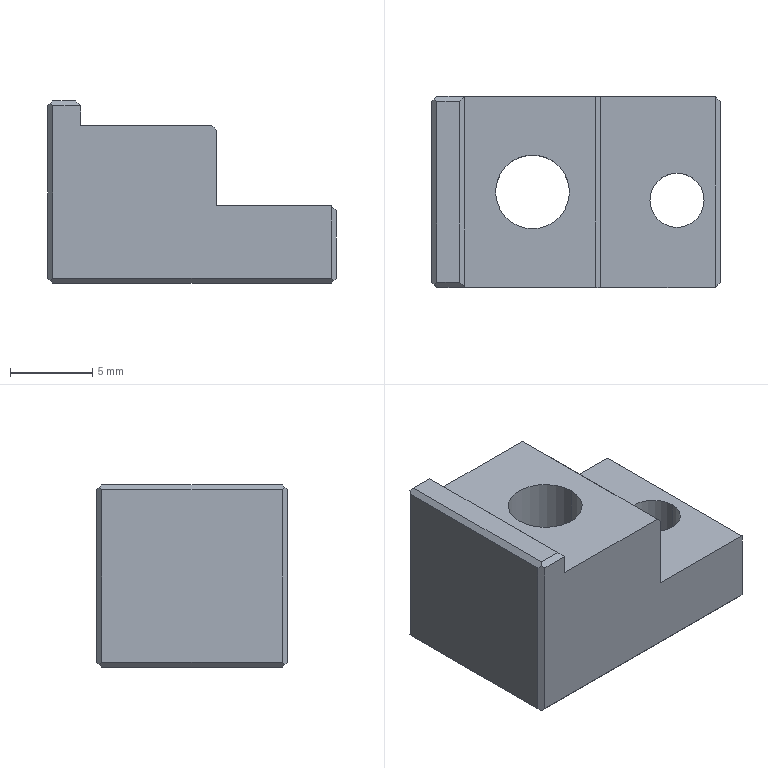Part | NX | 1 solid | 32 faces | box 17.581 x 11.62 x 11.1 mm | volume 1380 mm3 | plane 24 | cone 4 | cylinder 4 | commonest cylinder face diameters 3.3 x2 4.5 x2
STEP:
#1=CARTESIAN_POINT('',(1997.881,152.8,-124.5));
#2=VERTEX_POINT('',#1);
#3=CARTESIAN_POINT('',(1997.881,152.8,-128.6));
#4=VERTEX_POINT('',#3);
#5=CARTESIAN_POINT('',(1997.881,152.8,-126.55));
#6=DIRECTION('',(0.,0.,-1.));
#7=VECTOR('',#6,1000.);
#8=LINE('',#5,#7);
#9=EDGE_CURVE('',#2,#4,#8,.T.);
#10=ORIENTED_EDGE('',*,*,#9,.T.);
#11=CARTESIAN_POINT('',(1997.881,163.82,-128.6));
#12=VERTEX_POINT('',#11);
#13=CARTESIAN_POINT('',(1997.881,158.31,-128.6));
#14=DIRECTION('',(0.,1.,0.));
#15=VECTOR('',#14,1000.);
#16=LINE('',#13,#15);
#17=EDGE_CURVE('',#4,#12,#16,.T.);
#18=ORIENTED_EDGE('',*,*,#17,.T.);
#19=CARTESIAN_POINT('',(1997.881,163.82,-124.5));
#20=VERTEX_POINT('',#19);
#21=CARTESIAN_POINT('',(1997.881,163.82,-126.55));
#22=DIRECTION('',(0.,0.,-1.));
#23=VECTOR('',#22,1000.);
#24=LINE('',#21,#23);
#25=EDGE_CURVE('',#20,#12,#24,.T.);
#26=ORIENTED_EDGE('',*,*,#25,.F.);
#27=CARTESIAN_POINT('',(1997.881,158.31,-124.5));
#28=DIRECTION('',(0.,1.,0.));
#29=VECTOR('',#28,1000.);
#30=LINE('',#27,#29);
#31=EDGE_CURVE('',#2,#20,#30,.T.);
#32=ORIENTED_EDGE('',*,*,#31,.F.);
#33=EDGE_LOOP('',(#10,#18,#26,#32));
#34=FACE_BOUND('',#33,.T.);
#35=CARTESIAN_POINT('',(1997.881,144.5,-119.3));
#36=DIRECTION('',(1.,0.,0.));
#37=DIRECTION('',(0.,1.,0.));
#38=AXIS2_PLACEMENT_3D('',#35,#36,#37);
#39=PLANE('',#38);
#40=ADVANCED_FACE('',(#34),#39,.T.);
#41=CARTESIAN_POINT('',(1980.6,164.12,-128.6));
#42=VERTEX_POINT('',#41);
#43=CARTESIAN_POINT('',(1980.6,164.12,-118.1));
#44=VERTEX_POINT('',#43);
#45=CARTESIAN_POINT('',(1980.6,164.12,-123.35));
#46=DIRECTION('',(0.,0.,1.));
#47=VECTOR('',#46,1000.);
#48=LINE('',#45,#47);
#49=EDGE_CURVE('',#42,#44,#48,.T.);
#50=ORIENTED_EDGE('',*,*,#49,.T.);
#51=CARTESIAN_POINT('',(1982.3,164.12,-118.1));
#52=VERTEX_POINT('',#51);
#53=CARTESIAN_POINT('',(1981.3,164.12,-118.1));
#54=DIRECTION('',(-1.,0.,0.));
#55=VECTOR('',#54,1000.);
#56=LINE('',#53,#55);
#57=EDGE_CURVE('',#52,#44,#56,.T.);
#58=ORIENTED_EDGE('',*,*,#57,.F.);
#59=CARTESIAN_POINT('',(1982.3,164.12,-119.3));
#60=VERTEX_POINT('',#59);
#61=CARTESIAN_POINT('',(1982.3,164.12,-119.3));
#62=DIRECTION('',(0.,0.,1.));
#63=VECTOR('',#62,1000.);
#64=LINE('',#61,#63);
#65=EDGE_CURVE('',#60,#52,#64,.T.);
#66=ORIENTED_EDGE('',*,*,#65,.F.);
#67=CARTESIAN_POINT('',(1990.281,164.12,-119.3));
#68=VERTEX_POINT('',#67);
#69=CARTESIAN_POINT('',(1982.3,164.12,-119.3));
#70=DIRECTION('',(-1.,0.,0.));
#71=VECTOR('',#70,1000.);
#72=LINE('',#69,#71);
#73=EDGE_CURVE('',#68,#60,#72,.T.);
#74=ORIENTED_EDGE('',*,*,#73,.F.);
#75=CARTESIAN_POINT('',(1990.581,164.12,-119.6));
#76=VERTEX_POINT('',#75);
#77=CARTESIAN_POINT('',(1990.281,164.12,-119.3));
#78=DIRECTION('',(0.7071,0.,-0.7071));
#79=VECTOR('',#78,1000.);
#80=LINE('',#77,#79);
#81=EDGE_CURVE('',#68,#76,#80,.T.);
#82=ORIENTED_EDGE('',*,*,#81,.T.);
#83=CARTESIAN_POINT('',(1990.581,164.12,-124.2));
#84=VERTEX_POINT('',#83);
#85=CARTESIAN_POINT('',(1990.581,164.12,-119.3));
#86=DIRECTION('',(0.,0.,1.));
#87=VECTOR('',#86,1000.);
#88=LINE('',#85,#87);
#89=EDGE_CURVE('',#84,#76,#88,.T.);
#90=ORIENTED_EDGE('',*,*,#89,.F.);
#91=CARTESIAN_POINT('',(1997.581,164.12,-124.2));
#92=VERTEX_POINT('',#91);
#93=CARTESIAN_POINT('',(1997.8,164.12,-124.2));
#94=DIRECTION('',(-1.,0.,0.));
#95=VECTOR('',#94,1000.);
#96=LINE('',#93,#95);
#97=EDGE_CURVE('',#92,#84,#96,.T.);
#98=ORIENTED_EDGE('',*,*,#97,.F.);
#99=CARTESIAN_POINT('',(1997.581,164.12,-128.6));
#100=VERTEX_POINT('',#99);
#101=CARTESIAN_POINT('',(1997.581,164.12,-126.55));
#102=DIRECTION('',(0.,0.,-1.));
#103=VECTOR('',#102,1000.);
#104=LINE('',#101,#103);
#105=EDGE_CURVE('',#92,#100,#104,.T.);
#106=ORIENTED_EDGE('',*,*,#105,.T.);
#107=CARTESIAN_POINT('',(1989.09,164.12,-128.6));
#108=DIRECTION('',(-1.,0.,0.));
#109=VECTOR('',#108,1000.);
#110=LINE('',#107,#109);
#111=EDGE_CURVE('',#100,#42,#110,.T.);
#112=ORIENTED_EDGE('',*,*,#111,.T.);
#113=EDGE_LOOP('',(#50,#58,#66,#74,#82,#90,#98,#106,#112));
#114=FACE_BOUND('',#113,.T.);
#115=CARTESIAN_POINT('',(1980.3,164.12,-119.3));
#116=DIRECTION('',(0.,1.,0.));
#117=DIRECTION('',(1.,0.,0.));
#118=AXIS2_PLACEMENT_3D('',#115,#116,#117);
#119=PLANE('',#118);
#120=ADVANCED_FACE('',(#114),#119,.T.);
#121=CARTESIAN_POINT('',(1988.69,158.31,-128.7));
#122=VERTEX_POINT('',#121);
#123=CARTESIAN_POINT('',(1984.19,158.31,-128.7));
#124=VERTEX_POINT('',#123);
#125=CARTESIAN_POINT('',(1986.44,158.31,-128.7));
#126=DIRECTION('',(0.,0.,-1.));
#127=DIRECTION('',(-1.,0.,0.));
#128=AXIS2_PLACEMENT_3D('',#125,#126,#127);
#129=CIRCLE('',#128,2.25);
#130=EDGE_CURVE('',#122,#124,#129,.T.);
#131=ORIENTED_EDGE('',*,*,#130,.F.);
#132=CARTESIAN_POINT('',(1988.89,158.31,-128.9));
#133=VERTEX_POINT('',#132);
#134=CARTESIAN_POINT('',(1988.69,158.31,-128.7));
#135=DIRECTION('',(0.7071,0.,-0.7071));
#136=VECTOR('',#135,1000.);
#137=LINE('',#134,#136);
#138=EDGE_CURVE('',#133,#122,#137,.F.);
#139=ORIENTED_EDGE('',*,*,#138,.F.);
#140=CARTESIAN_POINT('',(1983.99,158.31,-128.9));
#141=VERTEX_POINT('',#140);
#142=CARTESIAN_POINT('',(1986.44,158.31,-128.9));
#143=DIRECTION('',(0.,0.,-1.));
#144=DIRECTION('',(-1.,0.,0.));
#145=AXIS2_PLACEMENT_3D('',#142,#143,#144);
#146=CIRCLE('',#145,2.45);
#147=EDGE_CURVE('',#133,#141,#146,.T.);
#148=ORIENTED_EDGE('',*,*,#147,.T.);
#149=CARTESIAN_POINT('',(1984.19,158.31,-128.7));
#150=DIRECTION('',(-0.7071,0.,-0.7071));
#151=VECTOR('',#150,1000.);
#152=LINE('',#149,#151);
#153=EDGE_CURVE('',#141,#124,#152,.F.);
#154=ORIENTED_EDGE('',*,*,#153,.T.);
#155=EDGE_LOOP('',(#131,#139,#148,#154));
#156=FACE_BOUND('',#155,.T.);
#157=CARTESIAN_POINT('',(1986.44,158.31,-128.7));
#158=DIRECTION('',(0.,0.,-1.));
#159=DIRECTION('',(-1.,0.,0.));
#160=AXIS2_PLACEMENT_3D('',#157,#158,#159);
#161=CONICAL_SURFACE('',#160,2.25,0.7854);
#162=ADVANCED_FACE('',(#156),#161,.F.);
#163=CARTESIAN_POINT('',(1982.3,152.5,-119.3));
#164=VERTEX_POINT('',#163);
#165=CARTESIAN_POINT('',(1982.3,152.5,-118.1));
#166=VERTEX_POINT('',#165);
#167=CARTESIAN_POINT('',(1982.3,152.5,-119.3));
#168=DIRECTION('',(0.,0.,1.));
#169=VECTOR('',#168,1000.);
#170=LINE('',#167,#169);
#171=EDGE_CURVE('',#164,#166,#170,.T.);
#172=ORIENTED_EDGE('',*,*,#171,.T.);
#173=CARTESIAN_POINT('',(1980.6,152.5,-118.1));
#174=VERTEX_POINT('',#173);
#175=CARTESIAN_POINT('',(1981.3,152.5,-118.1));
#176=DIRECTION('',(1.,0.,0.));
#177=VECTOR('',#176,1000.);
#178=LINE('',#175,#177);
#179=EDGE_CURVE('',#174,#166,#178,.T.);
#180=ORIENTED_EDGE('',*,*,#179,.F.);
#181=CARTESIAN_POINT('',(1980.6,152.5,-128.6));
#182=VERTEX_POINT('',#181);
#183=CARTESIAN_POINT('',(1980.6,152.5,-123.35));
#184=DIRECTION('',(0.,0.,1.));
#185=VECTOR('',#184,1000.);
#186=LINE('',#183,#185);
#187=EDGE_CURVE('',#182,#174,#186,.T.);
#188=ORIENTED_EDGE('',*,*,#187,.F.);
#189=CARTESIAN_POINT('',(1997.581,152.5,-128.6));
#190=VERTEX_POINT('',#189);
#191=CARTESIAN_POINT('',(1989.09,152.5,-128.6));
#192=DIRECTION('',(-1.,0.,0.));
#193=VECTOR('',#192,1000.);
#194=LINE('',#191,#193);
#195=EDGE_CURVE('',#190,#182,#194,.T.);
#196=ORIENTED_EDGE('',*,*,#195,.F.);
#197=CARTESIAN_POINT('',(1997.581,152.5,-124.2));
#198=VERTEX_POINT('',#197);
#199=CARTESIAN_POINT('',(1997.581,152.5,-126.55));
#200=DIRECTION('',(0.,0.,-1.));
#201=VECTOR('',#200,1000.);
#202=LINE('',#199,#201);
#203=EDGE_CURVE('',#198,#190,#202,.T.);
#204=ORIENTED_EDGE('',*,*,#203,.F.);
#205=CARTESIAN_POINT('',(1990.581,152.5,-124.2));
#206=VERTEX_POINT('',#205);
#207=CARTESIAN_POINT('',(1997.8,152.5,-124.2));
#208=DIRECTION('',(1.,0.,0.));
#209=VECTOR('',#208,1000.);
#210=LINE('',#207,#209);
#211=EDGE_CURVE('',#206,#198,#210,.T.);
#212=ORIENTED_EDGE('',*,*,#211,.F.);
#213=CARTESIAN_POINT('',(1990.581,152.5,-119.6));
#214=VERTEX_POINT('',#213);
#215=CARTESIAN_POINT('',(1990.581,152.5,-119.3));
#216=DIRECTION('',(0.,0.,-1.));
#217=VECTOR('',#216,1000.);
#218=LINE('',#215,#217);
#219=EDGE_CURVE('',#214,#206,#218,.T.);
#220=ORIENTED_EDGE('',*,*,#219,.F.);
#221=CARTESIAN_POINT('',(1990.281,152.5,-119.3));
#222=VERTEX_POINT('',#221);
#223=CARTESIAN_POINT('',(1990.281,152.5,-119.3));
#224=DIRECTION('',(-0.7071,0.,0.7071));
#225=VECTOR('',#224,1000.);
#226=LINE('',#223,#225);
#227=EDGE_CURVE('',#214,#222,#226,.T.);
#228=ORIENTED_EDGE('',*,*,#227,.T.);
#229=CARTESIAN_POINT('',(1988.678,152.5,-119.3));
#230=DIRECTION('',(-1.,0.,0.));
#231=VECTOR('',#230,1000.);
#232=LINE('',#229,#231);
#233=EDGE_CURVE('',#222,#164,#232,.T.);
#234=ORIENTED_EDGE('',*,*,#233,.T.);
#235=EDGE_LOOP('',(#172,#180,#188,#196,#204,#212,#220,#228,#234));
#236=FACE_BOUND('',#235,.T.);
#237=CARTESIAN_POINT('',(1982.3,152.5,-119.3));
#238=DIRECTION('',(0.,-1.,0.));
#239=DIRECTION('',(0.,0.,-1.));
#240=AXIS2_PLACEMENT_3D('',#237,#238,#239);
#241=PLANE('',#240);
#242=ADVANCED_FACE('',(#236),#241,.T.);
#243=ORIENTED_EDGE('',*,*,#130,.T.);
#244=CARTESIAN_POINT('',(1984.19,158.31,-119.3));
#245=VERTEX_POINT('',#244);
#246=CARTESIAN_POINT('',(1984.19,158.31,-128.9));
#247=DIRECTION('',(0.,0.,-1.));
#248=VECTOR('',#247,1000.);
#249=LINE('',#246,#248);
#250=EDGE_CURVE('',#124,#245,#249,.F.);
#251=ORIENTED_EDGE('',*,*,#250,.T.);
#252=CARTESIAN_POINT('',(1988.69,158.31,-119.3));
#253=VERTEX_POINT('',#252);
#254=CARTESIAN_POINT('',(1986.44,158.31,-119.3));
#255=DIRECTION('',(0.,0.,-1.));
#256=DIRECTION('',(-1.,0.,0.));
#257=AXIS2_PLACEMENT_3D('',#254,#255,#256);
#258=CIRCLE('',#257,2.25);
#259=EDGE_CURVE('',#253,#245,#258,.T.);
#260=ORIENTED_EDGE('',*,*,#259,.F.);
#261=CARTESIAN_POINT('',(1988.69,158.31,-128.9));
#262=DIRECTION('',(0.,0.,-1.));
#263=VECTOR('',#262,1000.);
#264=LINE('',#261,#263);
#265=EDGE_CURVE('',#122,#253,#264,.F.);
#266=ORIENTED_EDGE('',*,*,#265,.F.);
#267=EDGE_LOOP('',(#243,#251,#260,#266));
#268=FACE_BOUND('',#267,.T.);
#269=CARTESIAN_POINT('',(1986.44,158.31,-128.9));
#270=DIRECTION('',(0.,0.,-1.));
#271=DIRECTION('',(-1.,0.,0.));
#272=AXIS2_PLACEMENT_3D('',#269,#270,#271);
#273=CYLINDRICAL_SURFACE('',#272,2.25);
#274=ADVANCED_FACE('',(#268),#273,.F.);
#275=CARTESIAN_POINT('',(1982.,163.82,-117.8));
#276=VERTEX_POINT('',#275);
#277=CARTESIAN_POINT('',(1980.6,163.82,-117.8));
#278=VERTEX_POINT('',#277);
#279=CARTESIAN_POINT('',(1981.3,163.82,-117.8));
#280=DIRECTION('',(-1.,0.,0.));
#281=VECTOR('',#280,1000.);
#282=LINE('',#279,#281);
#283=EDGE_CURVE('',#276,#278,#282,.T.);
#284=ORIENTED_EDGE('',*,*,#283,.T.);
#285=CARTESIAN_POINT('',(1980.6,152.8,-117.8));
#286=VERTEX_POINT('',#285);
#287=CARTESIAN_POINT('',(1980.6,158.31,-117.8));
#288=DIRECTION('',(0.,-1.,0.));
#289=VECTOR('',#288,1000.);
#290=LINE('',#287,#289);
#291=EDGE_CURVE('',#278,#286,#290,.T.);
#292=ORIENTED_EDGE('',*,*,#291,.T.);
#293=CARTESIAN_POINT('',(1982.,152.8,-117.8));
#294=VERTEX_POINT('',#293);
#295=CARTESIAN_POINT('',(1981.3,152.8,-117.8));
#296=DIRECTION('',(1.,0.,0.));
#297=VECTOR('',#296,1000.);
#298=LINE('',#295,#297);
#299=EDGE_CURVE('',#286,#294,#298,.T.);
#300=ORIENTED_EDGE('',*,*,#299,.T.);
#301=CARTESIAN_POINT('',(1982.,158.31,-117.8));
#302=DIRECTION('',(0.,1.,0.));
#303=VECTOR('',#302,1000.);
#304=LINE('',#301,#303);
#305=EDGE_CURVE('',#294,#276,#304,.T.);
#306=ORIENTED_EDGE('',*,*,#305,.T.);
#307=EDGE_LOOP('',(#284,#292,#300,#306));
#308=FACE_BOUND('',#307,.T.);
#309=CARTESIAN_POINT('',(1989.636,158.31,-117.8));
#310=DIRECTION('',(0.,0.,1.));
#311=DIRECTION('',(1.,0.,0.));
#312=AXIS2_PLACEMENT_3D('',#309,#310,#311);
#313=PLANE('',#312);
#314=ADVANCED_FACE('',(#308),#313,.T.);
#315=CARTESIAN_POINT('',(1982.3,148.25,-119.3));
#316=DIRECTION('',(0.,-1.,0.));
#317=VECTOR('',#316,1000.);
#318=LINE('',#315,#317);
#319=EDGE_CURVE('',#60,#164,#318,.T.);
#320=ORIENTED_EDGE('',*,*,#319,.F.);
#321=ORIENTED_EDGE('',*,*,#65,.T.);
#322=CARTESIAN_POINT('',(1982.3,158.31,-118.1));
#323=DIRECTION('',(0.,1.,0.));
#324=VECTOR('',#323,1000.);
#325=LINE('',#322,#324);
#326=EDGE_CURVE('',#166,#52,#325,.T.);
#327=ORIENTED_EDGE('',*,*,#326,.F.);
#328=ORIENTED_EDGE('',*,*,#171,.F.);
#329=EDGE_LOOP('',(#320,#321,#327,#328));
#330=FACE_BOUND('',#329,.T.);
#331=CARTESIAN_POINT('',(1982.3,164.12,-119.3));
#332=DIRECTION('',(1.,0.,0.));
#333=DIRECTION('',(0.,1.,0.));
#334=AXIS2_PLACEMENT_3D('',#331,#332,#333);
#335=PLANE('',#334);
#336=ADVANCED_FACE('',(#330),#335,.T.);
#337=ORIENTED_EDGE('',*,*,#111,.F.);
#338=CARTESIAN_POINT('',(1997.731,163.97,-128.75));
#339=VERTEX_POINT('',#338);
#340=CARTESIAN_POINT('',(1988.281,173.42,-119.3));
#341=DIRECTION('',(-0.5774,0.5774,0.5774));
#342=VECTOR('',#341,1000.);
#343=LINE('',#340,#342);
#344=EDGE_CURVE('',#339,#100,#343,.T.);
#345=ORIENTED_EDGE('',*,*,#344,.F.);
#346=CARTESIAN_POINT('',(1997.581,163.82,-128.9));
#347=VERTEX_POINT('',#346);
#348=CARTESIAN_POINT('',(2007.181,173.42,-119.3));
#349=DIRECTION('',(0.5774,0.5774,0.5774));
#350=VECTOR('',#349,1000.);
#351=LINE('',#348,#350);
#352=EDGE_CURVE('',#347,#339,#351,.T.);
#353=ORIENTED_EDGE('',*,*,#352,.F.);
#354=CARTESIAN_POINT('',(1980.6,163.82,-128.9));
#355=VERTEX_POINT('',#354);
#356=CARTESIAN_POINT('',(1989.09,163.82,-128.9));
#357=DIRECTION('',(-1.,0.,0.));
#358=VECTOR('',#357,1000.);
#359=LINE('',#356,#358);
#360=EDGE_CURVE('',#347,#355,#359,.T.);
#361=ORIENTED_EDGE('',*,*,#360,.T.);
#362=CARTESIAN_POINT('',(1980.45,163.97,-128.75));
#363=VERTEX_POINT('',#362);
#364=CARTESIAN_POINT('',(1971.,173.42,-119.3));
#365=DIRECTION('',(-0.5774,0.5774,0.5774));
#366=VECTOR('',#365,1000.);
#367=LINE('',#364,#366);
#368=EDGE_CURVE('',#355,#363,#367,.T.);
#369=ORIENTED_EDGE('',*,*,#368,.T.);
#370=CARTESIAN_POINT('',(1989.9,173.42,-119.3));
#371=DIRECTION('',(0.5774,0.5774,0.5774));
#372=VECTOR('',#371,1000.);
#373=LINE('',#370,#372);
#374=EDGE_CURVE('',#363,#42,#373,.T.);
#375=ORIENTED_EDGE('',*,*,#374,.T.);
#376=EDGE_LOOP('',(#337,#345,#353,#361,#369,#375));
#377=FACE_BOUND('',#376,.T.);
#378=CARTESIAN_POINT('',(1989.09,163.97,-128.75));
#379=DIRECTION('',(0.,0.7071,-0.7071));
#380=DIRECTION('',(-1.,0.,0.));
#381=AXIS2_PLACEMENT_3D('',#378,#379,#380);
#382=PLANE('',#381);
#383=ADVANCED_FACE('',(#377),#382,.T.);
#384=ORIENTED_EDGE('',*,*,#25,.T.);
#385=CARTESIAN_POINT('',(2013.451,148.25,-113.03));
#386=DIRECTION('',(-0.5774,0.5774,-0.5774));
#387=VECTOR('',#386,1000.);
#388=LINE('',#385,#387);
#389=EDGE_CURVE('',#12,#339,#388,.T.);
#390=ORIENTED_EDGE('',*,*,#389,.T.);
#391=ORIENTED_EDGE('',*,*,#344,.T.);
#392=ORIENTED_EDGE('',*,*,#105,.F.);
#393=CARTESIAN_POINT('',(2013.451,148.25,-140.07));
#394=DIRECTION('',(0.5774,-0.5774,-0.5774));
#395=VECTOR('',#394,1000.);
#396=LINE('',#393,#395);
#397=EDGE_CURVE('',#92,#20,#396,.T.);
#398=ORIENTED_EDGE('',*,*,#397,.T.);
#399=EDGE_LOOP('',(#384,#390,#391,#392,#398));
#400=FACE_BOUND('',#399,.T.);
#401=CARTESIAN_POINT('',(1997.731,163.97,-126.55));
#402=DIRECTION('',(-0.7071,-0.7071,0.));
#403=DIRECTION('',(-0.7071,0.7071,0.));
#404=AXIS2_PLACEMENT_3D('',#401,#402,#403);
#405=PLANE('',#404);
#406=ADVANCED_FACE('',(#400),#405,.F.);
#407=ORIENTED_EDGE('',*,*,#9,.F.);
#408=CARTESIAN_POINT('',(1992.681,147.6,-119.3));
#409=DIRECTION('',(0.5774,0.5774,-0.5774));
#410=VECTOR('',#409,1000.);
#411=LINE('',#408,#410);
#412=EDGE_CURVE('',#198,#2,#411,.T.);
#413=ORIENTED_EDGE('',*,*,#412,.F.);
#414=ORIENTED_EDGE('',*,*,#203,.T.);
#415=CARTESIAN_POINT('',(1997.731,152.65,-128.75));
#416=VERTEX_POINT('',#415);
#417=CARTESIAN_POINT('',(1988.281,143.2,-119.3));
#418=DIRECTION('',(0.5774,0.5774,-0.5774));
#419=VECTOR('',#418,1000.);
#420=LINE('',#417,#419);
#421=EDGE_CURVE('',#190,#416,#420,.T.);
#422=ORIENTED_EDGE('',*,*,#421,.T.);
#423=CARTESIAN_POINT('',(2007.181,162.1,-119.3));
#424=DIRECTION('',(0.5774,0.5774,0.5774));
#425=VECTOR('',#424,1000.);
#426=LINE('',#423,#425);
#427=EDGE_CURVE('',#416,#4,#426,.T.);
#428=ORIENTED_EDGE('',*,*,#427,.T.);
#429=EDGE_LOOP('',(#407,#413,#414,#422,#428));
#430=FACE_BOUND('',#429,.T.);
#431=CARTESIAN_POINT('',(1997.731,152.65,-126.55));
#432=DIRECTION('',(0.7071,-0.7071,0.));
#433=DIRECTION('',(0.,0.,-1.));
#434=AXIS2_PLACEMENT_3D('',#431,#432,#433);
#435=PLANE('',#434);
#436=ADVANCED_FACE('',(#430),#435,.T.);
#437=ORIENTED_EDGE('',*,*,#49,.F.);
#438=ORIENTED_EDGE('',*,*,#374,.F.);
#439=CARTESIAN_POINT('',(1980.3,163.82,-128.6));
#440=VERTEX_POINT('',#439);
#441=CARTESIAN_POINT('',(1971.,154.52,-119.3));
#442=DIRECTION('',(0.5774,0.5774,-0.5774));
#443=VECTOR('',#442,1000.);
#444=LINE('',#441,#443);
#445=EDGE_CURVE('',#440,#363,#444,.T.);
#446=ORIENTED_EDGE('',*,*,#445,.F.);
#447=CARTESIAN_POINT('',(1980.3,163.82,-118.1));
#448=VERTEX_POINT('',#447);
#449=CARTESIAN_POINT('',(1980.3,163.82,-123.35));
#450=DIRECTION('',(0.,0.,1.));
#451=VECTOR('',#450,1000.);
#452=LINE('',#449,#451);
#453=EDGE_CURVE('',#440,#448,#452,.T.);
#454=ORIENTED_EDGE('',*,*,#453,.T.);
#455=CARTESIAN_POINT('',(1980.45,163.97,-117.95));
#456=VERTEX_POINT('',#455);
#457=CARTESIAN_POINT('',(1997.8,181.32,-100.6));
#458=DIRECTION('',(0.5774,0.5774,0.5774));
#459=VECTOR('',#458,1000.);
#460=LINE('',#457,#459);
#461=EDGE_CURVE('',#448,#456,#460,.T.);
#462=ORIENTED_EDGE('',*,*,#461,.T.);
#463=CARTESIAN_POINT('',(1964.73,148.25,-102.23));
#464=DIRECTION('',(0.5774,0.5774,-0.5774));
#465=VECTOR('',#464,1000.);
#466=LINE('',#463,#465);
#467=EDGE_CURVE('',#456,#44,#466,.T.);
#468=ORIENTED_EDGE('',*,*,#467,.T.);
#469=EDGE_LOOP('',(#437,#438,#446,#454,#462,#468));
#470=FACE_BOUND('',#469,.T.);
#471=CARTESIAN_POINT('',(1980.45,163.97,-123.35));
#472=DIRECTION('',(-0.7071,0.7071,0.));
#473=DIRECTION('',(0.,0.,1.));
#474=AXIS2_PLACEMENT_3D('',#471,#472,#473);
#475=PLANE('',#474);
#476=ADVANCED_FACE('',(#470),#475,.T.);
#477=ORIENTED_EDGE('',*,*,#291,.F.);
#478=CARTESIAN_POINT('',(1996.17,148.25,-102.23));
#479=DIRECTION('',(-0.5774,0.5774,-0.5774));
#480=VECTOR('',#479,1000.);
#481=LINE('',#478,#480);
#482=EDGE_CURVE('',#278,#456,#481,.T.);
#483=ORIENTED_EDGE('',*,*,#482,.T.);
#484=ORIENTED_EDGE('',*,*,#461,.F.);
#485=CARTESIAN_POINT('',(1980.3,152.8,-118.1));
#486=VERTEX_POINT('',#485);
#487=CARTESIAN_POINT('',(1980.3,158.31,-118.1));
#488=DIRECTION('',(0.,-1.,0.));
#489=VECTOR('',#488,1000.);
#490=LINE('',#487,#489);
#491=EDGE_CURVE('',#448,#486,#490,.T.);
#492=ORIENTED_EDGE('',*,*,#491,.T.);
#493=CARTESIAN_POINT('',(1980.45,152.65,-117.95));
#494=VERTEX_POINT('',#493);
#495=CARTESIAN_POINT('',(1997.8,135.3,-100.6));
#496=DIRECTION('',(-0.5774,0.5774,-0.5774));
#497=VECTOR('',#496,1000.);
#498=LINE('',#495,#497);
#499=EDGE_CURVE('',#494,#486,#498,.T.);
#500=ORIENTED_EDGE('',*,*,#499,.F.);
#501=CARTESIAN_POINT('',(1997.8,170.,-100.6));
#502=DIRECTION('',(0.5774,0.5774,0.5774));
#503=VECTOR('',#502,1000.);
#504=LINE('',#501,#503);
#505=EDGE_CURVE('',#494,#286,#504,.T.);
#506=ORIENTED_EDGE('',*,*,#505,.T.);
#507=EDGE_LOOP('',(#477,#483,#484,#492,#500,#506));
#508=FACE_BOUND('',#507,.T.);
#509=CARTESIAN_POINT('',(1980.45,158.31,-117.95));
#510=DIRECTION('',(-0.7071,0.,0.7071));
#511=DIRECTION('',(0.,1.,0.));
#512=AXIS2_PLACEMENT_3D('',#509,#510,#511);
#513=PLANE('',#512);
#514=ADVANCED_FACE('',(#508),#513,.T.);
#515=ORIENTED_EDGE('',*,*,#305,.F.);
#516=CARTESIAN_POINT('',(1997.8,137.,-133.6));
#517=DIRECTION('',(0.5774,-0.5774,-0.5774));
#518=VECTOR('',#517,1000.);
#519=LINE('',#516,#518);
#520=EDGE_CURVE('',#294,#166,#519,.T.);
#521=ORIENTED_EDGE('',*,*,#520,.T.);
#522=ORIENTED_EDGE('',*,*,#326,.T.);
#523=CARTESIAN_POINT('',(1966.43,148.25,-102.23));
#524=DIRECTION('',(-0.5774,-0.5774,0.5774));
#525=VECTOR('',#524,1000.);
#526=LINE('',#523,#525);
#527=EDGE_CURVE('',#52,#276,#526,.T.);
#528=ORIENTED_EDGE('',*,*,#527,.T.);
#529=EDGE_LOOP('',(#515,#521,#522,#528));
#530=FACE_BOUND('',#529,.T.);
#531=CARTESIAN_POINT('',(1982.15,158.31,-117.95));
#532=DIRECTION('',(0.7071,0.,0.7071));
#533=DIRECTION('',(0.,-1.,0.));
#534=AXIS2_PLACEMENT_3D('',#531,#532,#533);
#535=PLANE('',#534);
#536=ADVANCED_FACE('',(#530),#535,.T.);
#537=ORIENTED_EDGE('',*,*,#299,.F.);
#538=ORIENTED_EDGE('',*,*,#505,.F.);
#539=CARTESIAN_POINT('',(1981.8,151.3,-119.3));
#540=DIRECTION('',(-0.5774,0.5774,0.5774));
#541=VECTOR('',#540,1000.);
#542=LINE('',#539,#541);
#543=EDGE_CURVE('',#174,#494,#542,.T.);
#544=ORIENTED_EDGE('',*,*,#543,.F.);
#545=ORIENTED_EDGE('',*,*,#179,.T.);
#546=ORIENTED_EDGE('',*,*,#520,.F.);
#547=EDGE_LOOP('',(#537,#538,#544,#545,#546));
#548=FACE_BOUND('',#547,.T.);
#549=CARTESIAN_POINT('',(1981.3,152.65,-117.95));
#550=DIRECTION('',(0.,-0.7071,0.7071));
#551=DIRECTION('',(-1.,0.,0.));
#552=AXIS2_PLACEMENT_3D('',#549,#550,#551);
#553=PLANE('',#552);
#554=ADVANCED_FACE('',(#548),#553,.T.);
#555=ORIENTED_EDGE('',*,*,#283,.F.);
#556=ORIENTED_EDGE('',*,*,#527,.F.);
#557=ORIENTED_EDGE('',*,*,#57,.T.);
#558=ORIENTED_EDGE('',*,*,#467,.F.);
#559=ORIENTED_EDGE('',*,*,#482,.F.);
#560=EDGE_LOOP('',(#555,#556,#557,#558,#559));
#561=FACE_BOUND('',#560,.T.);
#562=CARTESIAN_POINT('',(1981.3,163.97,-117.95));
#563=DIRECTION('',(0.,0.7071,0.7071));
#564=DIRECTION('',(1.,0.,0.));
#565=AXIS2_PLACEMENT_3D('',#562,#563,#564);
#566=PLANE('',#565);
#567=ADVANCED_FACE('',(#561),#566,.T.);
#568=ORIENTED_EDGE('',*,*,#153,.F.);
#569=CARTESIAN_POINT('',(1986.44,158.31,-128.9));
#570=DIRECTION('',(0.,0.,-1.));
#571=DIRECTION('',(-1.,0.,0.));
#572=AXIS2_PLACEMENT_3D('',#569,#570,#571);
#573=CIRCLE('',#572,2.45);
#574=EDGE_CURVE('',#141,#133,#573,.T.);
#575=ORIENTED_EDGE('',*,*,#574,.T.);
#576=ORIENTED_EDGE('',*,*,#138,.T.);
#577=CARTESIAN_POINT('',(1986.44,158.31,-128.7));
#578=DIRECTION('',(0.,0.,-1.));
#579=DIRECTION('',(-1.,0.,0.));
#580=AXIS2_PLACEMENT_3D('',#577,#578,#579);
#581=CIRCLE('',#580,2.25);
#582=EDGE_CURVE('',#124,#122,#581,.T.);
#583=ORIENTED_EDGE('',*,*,#582,.F.);
#584=EDGE_LOOP('',(#568,#575,#576,#583));
#585=FACE_BOUND('',#584,.T.);
#586=CARTESIAN_POINT('',(1986.44,158.31,-128.7));
#587=DIRECTION('',(0.,0.,-1.));
#588=DIRECTION('',(-1.,0.,0.));
#589=AXIS2_PLACEMENT_3D('',#586,#587,#588);
#590=CONICAL_SURFACE('',#589,2.25,0.7854);
#591=ADVANCED_FACE('',(#585),#590,.F.);
#592=ORIENTED_EDGE('',*,*,#250,.F.);
#593=ORIENTED_EDGE('',*,*,#582,.T.);
#594=ORIENTED_EDGE('',*,*,#265,.T.);
#595=CARTESIAN_POINT('',(1986.44,158.31,-119.3));
#596=DIRECTION('',(0.,0.,-1.));
#597=DIRECTION('',(-1.,0.,0.));
#598=AXIS2_PLACEMENT_3D('',#595,#596,#597);
#599=CIRCLE('',#598,2.25);
#600=EDGE_CURVE('',#245,#253,#599,.T.);
#601=ORIENTED_EDGE('',*,*,#600,.F.);
#602=EDGE_LOOP('',(#592,#593,#594,#601));
#603=FACE_BOUND('',#602,.T.);
#604=CARTESIAN_POINT('',(1986.44,158.31,-128.9));
#605=DIRECTION('',(0.,0.,-1.));
#606=DIRECTION('',(-1.,0.,0.));
#607=AXIS2_PLACEMENT_3D('',#604,#605,#606);
#608=CYLINDRICAL_SURFACE('',#607,2.25);
#609=ADVANCED_FACE('',(#603),#608,.F.);
#610=CARTESIAN_POINT('',(1997.581,152.8,-128.9));
#611=VERTEX_POINT('',#610);
#612=CARTESIAN_POINT('',(1980.6,152.8,-128.9));
#613=VERTEX_POINT('',#612);
#614=CARTESIAN_POINT('',(1989.09,152.8,-128.9));
#615=DIRECTION('',(-1.,0.,0.));
#616=VECTOR('',#615,1000.);
#617=LINE('',#614,#616);
#618=EDGE_CURVE('',#611,#613,#617,.T.);
#619=ORIENTED_EDGE('',*,*,#618,.T.);
#620=CARTESIAN_POINT('',(1980.6,158.31,-128.9));
#621=DIRECTION('',(0.,-1.,0.));
#622=VECTOR('',#621,1000.);
#623=LINE('',#620,#622);
#624=EDGE_CURVE('',#355,#613,#623,.T.);
#625=ORIENTED_EDGE('',*,*,#624,.F.);
#626=ORIENTED_EDGE('',*,*,#360,.F.);
#627=CARTESIAN_POINT('',(1997.581,158.31,-128.9));
#628=DIRECTION('',(0.,1.,0.));
#629=VECTOR('',#628,1000.);
#630=LINE('',#627,#629);
#631=EDGE_CURVE('',#611,#347,#630,.T.);
#632=ORIENTED_EDGE('',*,*,#631,.F.);
#633=EDGE_LOOP('',(#619,#625,#626,#632));
#634=FACE_BOUND('',#633,.T.);
#635=ORIENTED_EDGE('',*,*,#147,.F.);
#636=ORIENTED_EDGE('',*,*,#574,.F.);
#637=EDGE_LOOP('',(#635,#636));
#638=FACE_BOUND('',#637,.T.);
#639=CARTESIAN_POINT('',(1997.559,157.81,-128.9));
#640=VERTEX_POINT('',#639);
#641=CARTESIAN_POINT('',(1992.929,157.81,-128.9));
#642=VERTEX_POINT('',#641);
#643=CARTESIAN_POINT('',(1995.244,157.81,-128.9));
#644=DIRECTION('',(0.,0.,-1.));
#645=DIRECTION('',(-1.,0.,0.));
#646=AXIS2_PLACEMENT_3D('',#643,#644,#645);
#647=CIRCLE('',#646,2.315);
#648=EDGE_CURVE('',#640,#642,#647,.T.);
#649=ORIENTED_EDGE('',*,*,#648,.F.);
#650=CARTESIAN_POINT('',(1995.244,157.81,-128.9));
#651=DIRECTION('',(0.,0.,-1.));
#652=DIRECTION('',(-1.,0.,0.));
#653=AXIS2_PLACEMENT_3D('',#650,#651,#652);
#654=CIRCLE('',#653,2.315);
#655=EDGE_CURVE('',#642,#640,#654,.T.);
#656=ORIENTED_EDGE('',*,*,#655,.F.);
#657=EDGE_LOOP('',(#649,#656));
#658=FACE_BOUND('',#657,.T.);
#659=CARTESIAN_POINT('',(1997.8,148.25,-128.9));
#660=DIRECTION('',(0.,0.,-1.));
#661=DIRECTION('',(0.,-1.,0.));
#662=AXIS2_PLACEMENT_3D('',#659,#660,#661);
#663=PLANE('',#662);
#664=ADVANCED_FACE('',(#634,#638,#658),#663,.T.);
#665=ORIENTED_EDGE('',*,*,#631,.T.);
#666=ORIENTED_EDGE('',*,*,#352,.T.);
#667=ORIENTED_EDGE('',*,*,#389,.F.);
#668=ORIENTED_EDGE('',*,*,#17,.F.);
#669=ORIENTED_EDGE('',*,*,#427,.F.);
#670=CARTESIAN_POINT('',(2007.181,143.2,-119.3));
#671=DIRECTION('',(0.5774,-0.5774,0.5774));
#672=VECTOR('',#671,1000.);
#673=LINE('',#670,#672);
#674=EDGE_CURVE('',#611,#416,#673,.T.);
#675=ORIENTED_EDGE('',*,*,#674,.F.);
#676=EDGE_LOOP('',(#665,#666,#667,#668,#669,#675));
#677=FACE_BOUND('',#676,.T.);
#678=CARTESIAN_POINT('',(1997.731,158.31,-128.75));
#679=DIRECTION('',(-0.7071,0.,0.7071));
#680=DIRECTION('',(0.,1.,0.));
#681=AXIS2_PLACEMENT_3D('',#678,#679,#680);
#682=PLANE('',#681);
#683=ADVANCED_FACE('',(#677),#682,.F.);
#684=ORIENTED_EDGE('',*,*,#618,.F.);
#685=ORIENTED_EDGE('',*,*,#674,.T.);
#686=ORIENTED_EDGE('',*,*,#421,.F.);
#687=ORIENTED_EDGE('',*,*,#195,.T.);
#688=CARTESIAN_POINT('',(1980.45,152.65,-128.75));
#689=VERTEX_POINT('',#688);
#690=CARTESIAN_POINT('',(1989.9,143.2,-119.3));
#691=DIRECTION('',(-0.5774,0.5774,-0.5774));
#692=VECTOR('',#691,1000.);
#693=LINE('',#690,#692);
#694=EDGE_CURVE('',#182,#689,#693,.T.);
#695=ORIENTED_EDGE('',*,*,#694,.T.);
#696=CARTESIAN_POINT('',(1971.,143.2,-119.3));
#697=DIRECTION('',(0.5774,0.5774,-0.5774));
#698=VECTOR('',#697,1000.);
#699=LINE('',#696,#698);
#700=EDGE_CURVE('',#689,#613,#699,.T.);
#701=ORIENTED_EDGE('',*,*,#700,.T.);
#702=EDGE_LOOP('',(#684,#685,#686,#687,#695,#701));
#703=FACE_BOUND('',#702,.T.);
#704=CARTESIAN_POINT('',(1989.09,152.65,-128.75));
#705=DIRECTION('',(0.,-0.7071,-0.7071));
#706=DIRECTION('',(0.,0.7071,-0.7071));
#707=AXIS2_PLACEMENT_3D('',#704,#705,#706);
#708=PLANE('',#707);
#709=ADVANCED_FACE('',(#703),#708,.T.);
#710=CARTESIAN_POINT('',(1980.3,152.8,-128.6));
#711=VERTEX_POINT('',#710);
#712=CARTESIAN_POINT('',(1980.3,152.8,-123.35));
#713=DIRECTION('',(0.,0.,1.));
#714=VECTOR('',#713,1000.);
#715=LINE('',#712,#714);
#716=EDGE_CURVE('',#711,#486,#715,.T.);
#717=ORIENTED_EDGE('',*,*,#716,.T.);
#718=ORIENTED_EDGE('',*,*,#491,.F.);
#719=ORIENTED_EDGE('',*,*,#453,.F.);
#720=CARTESIAN_POINT('',(1980.3,158.31,-128.6));
#721=DIRECTION('',(0.,-1.,0.));
#722=VECTOR('',#721,1000.);
#723=LINE('',#720,#722);
#724=EDGE_CURVE('',#440,#711,#723,.T.);
#725=ORIENTED_EDGE('',*,*,#724,.T.);
#726=EDGE_LOOP('',(#717,#718,#719,#725));
#727=FACE_BOUND('',#726,.T.);
#728=CARTESIAN_POINT('',(1980.3,164.12,-119.3));
#729=DIRECTION('',(-1.,0.,0.));
#730=DIRECTION('',(0.,0.,1.));
#731=AXIS2_PLACEMENT_3D('',#728,#729,#730);
#732=PLANE('',#731);
#733=ADVANCED_FACE('',(#727),#732,.T.);
#734=ORIENTED_EDGE('',*,*,#724,.F.);
#735=ORIENTED_EDGE('',*,*,#445,.T.);
#736=ORIENTED_EDGE('',*,*,#368,.F.);
#737=ORIENTED_EDGE('',*,*,#624,.T.);
#738=ORIENTED_EDGE('',*,*,#700,.F.);
#739=CARTESIAN_POINT('',(1971.,162.1,-119.3));
#740=DIRECTION('',(-0.5774,0.5774,0.5774));
#741=VECTOR('',#740,1000.);
#742=LINE('',#739,#741);
#743=EDGE_CURVE('',#689,#711,#742,.T.);
#744=ORIENTED_EDGE('',*,*,#743,.T.);
#745=EDGE_LOOP('',(#734,#735,#736,#737,#738,#744));
#746=FACE_BOUND('',#745,.T.);
#747=CARTESIAN_POINT('',(1980.45,158.31,-128.75));
#748=DIRECTION('',(-0.7071,0.,-0.7071));
#749=DIRECTION('',(-0.7071,0.,0.7071));
#750=AXIS2_PLACEMENT_3D('',#747,#748,#749);
#751=PLANE('',#750);
#752=ADVANCED_FACE('',(#746),#751,.T.);
#753=ORIENTED_EDGE('',*,*,#716,.F.);
#754=ORIENTED_EDGE('',*,*,#743,.F.);
#755=ORIENTED_EDGE('',*,*,#694,.F.);
#756=ORIENTED_EDGE('',*,*,#187,.T.);
#757=ORIENTED_EDGE('',*,*,#543,.T.);
#758=ORIENTED_EDGE('',*,*,#499,.T.);
#759=EDGE_LOOP('',(#753,#754,#755,#756,#757,#758));
#760=FACE_BOUND('',#759,.T.);
#761=CARTESIAN_POINT('',(1980.45,152.65,-123.35));
#762=DIRECTION('',(-0.7071,-0.7071,0.));
#763=DIRECTION('',(-0.7071,0.7071,0.));
#764=AXIS2_PLACEMENT_3D('',#761,#762,#763);
#765=PLANE('',#764);
#766=ADVANCED_FACE('',(#760),#765,.T.);
#767=ORIENTED_EDGE('',*,*,#319,.T.);
#768=ORIENTED_EDGE('',*,*,#233,.F.);
#769=CARTESIAN_POINT('',(1990.281,158.31,-119.3));
#770=DIRECTION('',(0.,1.,0.));
#771=VECTOR('',#770,1000.);
#772=LINE('',#769,#771);
#773=EDGE_CURVE('',#222,#68,#772,.T.);
#774=ORIENTED_EDGE('',*,*,#773,.T.);
#775=ORIENTED_EDGE('',*,*,#73,.T.);
#776=EDGE_LOOP('',(#767,#768,#774,#775));
#777=FACE_BOUND('',#776,.T.);
#778=ORIENTED_EDGE('',*,*,#259,.T.);
#779=ORIENTED_EDGE('',*,*,#600,.T.);
#780=EDGE_LOOP('',(#778,#779));
#781=FACE_BOUND('',#780,.T.);
#782=CARTESIAN_POINT('',(1997.8,148.25,-119.3));
#783=DIRECTION('',(0.,0.,-1.));
#784=DIRECTION('',(0.,-1.,0.));
#785=AXIS2_PLACEMENT_3D('',#782,#783,#784);
#786=PLANE('',#785);
#787=ADVANCED_FACE('',(#777,#781),#786,.F.);
#788=CARTESIAN_POINT('',(1990.581,158.31,-119.6));
#789=DIRECTION('',(0.,1.,0.));
#790=VECTOR('',#789,1000.);
#791=LINE('',#788,#790);
#792=EDGE_CURVE('',#214,#76,#791,.T.);
#793=ORIENTED_EDGE('',*,*,#792,.F.);
#794=ORIENTED_EDGE('',*,*,#219,.T.);
#795=CARTESIAN_POINT('',(1990.581,148.038,-124.2));
#796=DIRECTION('',(0.,1.,0.));
#797=VECTOR('',#796,1000.);
#798=LINE('',#795,#797);
#799=EDGE_CURVE('',#206,#84,#798,.T.);
#800=ORIENTED_EDGE('',*,*,#799,.T.);
#801=ORIENTED_EDGE('',*,*,#89,.T.);
#802=EDGE_LOOP('',(#793,#794,#800,#801));
#803=FACE_BOUND('',#802,.T.);
#804=CARTESIAN_POINT('',(1990.581,148.038,-119.3));
#805=DIRECTION('',(-1.,0.,0.));
#806=DIRECTION('',(0.,0.,1.));
#807=AXIS2_PLACEMENT_3D('',#804,#805,#806);
#808=PLANE('',#807);
#809=ADVANCED_FACE('',(#803),#808,.F.);
#810=CARTESIAN_POINT('',(1997.581,158.31,-124.2));
#811=DIRECTION('',(0.,1.,0.));
#812=VECTOR('',#811,1000.);
#813=LINE('',#810,#812);
#814=EDGE_CURVE('',#198,#92,#813,.T.);
#815=ORIENTED_EDGE('',*,*,#814,.T.);
#816=ORIENTED_EDGE('',*,*,#97,.T.);
#817=ORIENTED_EDGE('',*,*,#799,.F.);
#818=ORIENTED_EDGE('',*,*,#211,.T.);
#819=EDGE_LOOP('',(#815,#816,#817,#818));
#820=FACE_BOUND('',#819,.T.);
#821=CARTESIAN_POINT('',(1996.894,157.81,-124.2));
#822=VERTEX_POINT('',#821);
#823=CARTESIAN_POINT('',(1993.594,157.81,-124.2));
#824=VERTEX_POINT('',#823);
#825=CARTESIAN_POINT('',(1995.244,157.81,-124.2));
#826=DIRECTION('',(0.,0.,-1.));
#827=DIRECTION('',(-1.,0.,0.));
#828=AXIS2_PLACEMENT_3D('',#825,#826,#827);
#829=CIRCLE('',#828,1.65);
#830=EDGE_CURVE('',#822,#824,#829,.T.);
#831=ORIENTED_EDGE('',*,*,#830,.T.);
#832=CARTESIAN_POINT('',(1995.244,157.81,-124.2));
#833=DIRECTION('',(0.,0.,-1.));
#834=DIRECTION('',(-1.,0.,0.));
#835=AXIS2_PLACEMENT_3D('',#832,#833,#834);
#836=CIRCLE('',#835,1.65);
#837=EDGE_CURVE('',#824,#822,#836,.T.);
#838=ORIENTED_EDGE('',*,*,#837,.T.);
#839=EDGE_LOOP('',(#831,#838));
#840=FACE_BOUND('',#839,.T.);
#841=CARTESIAN_POINT('',(1990.581,148.038,-124.2));
#842=DIRECTION('',(0.,0.,-1.));
#843=DIRECTION('',(0.,-1.,0.));
#844=AXIS2_PLACEMENT_3D('',#841,#842,#843);
#845=PLANE('',#844);
#846=ADVANCED_FACE('',(#820,#840),#845,.F.);
#847=CARTESIAN_POINT('',(1996.894,157.81,-128.516));
#848=VERTEX_POINT('',#847);
#849=CARTESIAN_POINT('',(1993.594,157.81,-128.516));
#850=VERTEX_POINT('',#849);
#851=CARTESIAN_POINT('',(1995.244,157.81,-128.516));
#852=DIRECTION('',(0.,0.,-1.));
#853=DIRECTION('',(-1.,0.,0.));
#854=AXIS2_PLACEMENT_3D('',#851,#852,#853);
#855=CIRCLE('',#854,1.65);
#856=EDGE_CURVE('',#848,#850,#855,.T.);
#857=ORIENTED_EDGE('',*,*,#856,.T.);
#858=CARTESIAN_POINT('',(1993.594,157.81,-128.9));
#859=DIRECTION('',(0.,0.,-1.));
#860=VECTOR('',#859,1000.);
#861=LINE('',#858,#860);
#862=EDGE_CURVE('',#850,#824,#861,.F.);
#863=ORIENTED_EDGE('',*,*,#862,.T.);
#864=ORIENTED_EDGE('',*,*,#830,.F.);
#865=CARTESIAN_POINT('',(1996.894,157.81,-128.9));
#866=DIRECTION('',(0.,0.,-1.));
#867=VECTOR('',#866,1000.);
#868=LINE('',#865,#867);
#869=EDGE_CURVE('',#848,#822,#868,.F.);
#870=ORIENTED_EDGE('',*,*,#869,.F.);
#871=EDGE_LOOP('',(#857,#863,#864,#870));
#872=FACE_BOUND('',#871,.T.);
#873=CARTESIAN_POINT('',(1995.244,157.81,-128.9));
#874=DIRECTION('',(0.,0.,-1.));
#875=DIRECTION('',(-1.,0.,0.));
#876=AXIS2_PLACEMENT_3D('',#873,#874,#875);
#877=CYLINDRICAL_SURFACE('',#876,1.65);
#878=ADVANCED_FACE('',(#872),#877,.F.);
#879=ORIENTED_EDGE('',*,*,#856,.F.);
#880=CARTESIAN_POINT('',(1996.894,157.81,-128.516));
#881=DIRECTION('',(0.866,0.,-0.5));
#882=VECTOR('',#881,1000.);
#883=LINE('',#880,#882);
#884=EDGE_CURVE('',#640,#848,#883,.F.);
#885=ORIENTED_EDGE('',*,*,#884,.F.);
#886=ORIENTED_EDGE('',*,*,#648,.T.);
#887=CARTESIAN_POINT('',(1993.594,157.81,-128.516));
#888=DIRECTION('',(-0.866,0.,-0.5));
#889=VECTOR('',#888,1000.);
#890=LINE('',#887,#889);
#891=EDGE_CURVE('',#642,#850,#890,.F.);
#892=ORIENTED_EDGE('',*,*,#891,.T.);
#893=EDGE_LOOP('',(#879,#885,#886,#892));
#894=FACE_BOUND('',#893,.T.);
#895=CARTESIAN_POINT('',(1995.244,157.81,-128.516));
#896=DIRECTION('',(0.,0.,-1.));
#897=DIRECTION('',(-1.,0.,0.));
#898=AXIS2_PLACEMENT_3D('',#895,#896,#897);
#899=CONICAL_SURFACE('',#898,1.65,1.047);
#900=ADVANCED_FACE('',(#894),#899,.F.);
#901=ORIENTED_EDGE('',*,*,#792,.T.);
#902=ORIENTED_EDGE('',*,*,#81,.F.);
#903=ORIENTED_EDGE('',*,*,#773,.F.);
#904=ORIENTED_EDGE('',*,*,#227,.F.);
#905=EDGE_LOOP('',(#901,#902,#903,#904));
#906=FACE_BOUND('',#905,.T.);
#907=CARTESIAN_POINT('',(1990.431,158.31,-119.45));
#908=DIRECTION('',(-0.7071,0.,-0.7071));
#909=DIRECTION('',(-0.7071,0.,0.7071));
#910=AXIS2_PLACEMENT_3D('',#907,#908,#909);
#911=PLANE('',#910);
#912=ADVANCED_FACE('',(#906),#911,.F.);
#913=ORIENTED_EDGE('',*,*,#814,.F.);
#914=ORIENTED_EDGE('',*,*,#412,.T.);
#915=ORIENTED_EDGE('',*,*,#31,.T.);
#916=ORIENTED_EDGE('',*,*,#397,.F.);
#917=EDGE_LOOP('',(#913,#914,#915,#916));
#918=FACE_BOUND('',#917,.T.);
#919=CARTESIAN_POINT('',(1997.731,158.31,-124.35));
#920=DIRECTION('',(0.7071,0.,0.7071));
#921=DIRECTION('',(0.,-1.,0.));
#922=AXIS2_PLACEMENT_3D('',#919,#920,#921);
#923=PLANE('',#922);
#924=ADVANCED_FACE('',(#918),#923,.T.);
#925=ORIENTED_EDGE('',*,*,#862,.F.);
#926=CARTESIAN_POINT('',(1995.244,157.81,-128.516));
#927=DIRECTION('',(0.,0.,-1.));
#928=DIRECTION('',(-1.,0.,0.));
#929=AXIS2_PLACEMENT_3D('',#926,#927,#928);
#930=CIRCLE('',#929,1.65);
#931=EDGE_CURVE('',#850,#848,#930,.T.);
#932=ORIENTED_EDGE('',*,*,#931,.T.);
#933=ORIENTED_EDGE('',*,*,#869,.T.);
#934=ORIENTED_EDGE('',*,*,#837,.F.);
#935=EDGE_LOOP('',(#925,#932,#933,#934));
#936=FACE_BOUND('',#935,.T.);
#937=CARTESIAN_POINT('',(1995.244,157.81,-128.9));
#938=DIRECTION('',(0.,0.,-1.));
#939=DIRECTION('',(-1.,0.,0.));
#940=AXIS2_PLACEMENT_3D('',#937,#938,#939);
#941=CYLINDRICAL_SURFACE('',#940,1.65);
#942=ADVANCED_FACE('',(#936),#941,.F.);
#943=ORIENTED_EDGE('',*,*,#891,.F.);
#944=ORIENTED_EDGE('',*,*,#655,.T.);
#945=ORIENTED_EDGE('',*,*,#884,.T.);
#946=ORIENTED_EDGE('',*,*,#931,.F.);
#947=EDGE_LOOP('',(#943,#944,#945,#946));
#948=FACE_BOUND('',#947,.T.);
#949=CARTESIAN_POINT('',(1995.244,157.81,-128.516));
#950=DIRECTION('',(0.,0.,-1.));
#951=DIRECTION('',(-1.,0.,0.));
#952=AXIS2_PLACEMENT_3D('',#949,#950,#951);
#953=CONICAL_SURFACE('',#952,1.65,1.047);
#954=ADVANCED_FACE('',(#948),#953,.F.);
#955=CLOSED_SHELL('',(#40,#120,#162,#242,#274,#314,#336,#383,#406,#436,#476,#514,#536,#554,#567,#591,#609,#664,#683,#709,#733,#752,#766,#787,#809,#846,#878,#900,#912,#924,#942,#954));
#956=MANIFOLD_SOLID_BREP('',#955);
#957=(LENGTH_UNIT()NAMED_UNIT(*)SI_UNIT(.MILLI.,.METRE.));
#958=UNCERTAINTY_MEASURE_WITH_UNIT(LENGTH_MEASURE(0.00001),#957,'','');
#959=(NAMED_UNIT(*)PLANE_ANGLE_UNIT()SI_UNIT($,.RADIAN.));
#960=(NAMED_UNIT(*)SI_UNIT($,.STERADIAN.)SOLID_ANGLE_UNIT());
#961=(GEOMETRIC_REPRESENTATION_CONTEXT(3)GLOBAL_UNCERTAINTY_ASSIGNED_CONTEXT((#958))GLOBAL_UNIT_ASSIGNED_CONTEXT((#957,#959,#960))REPRESENTATION_CONTEXT('',''));
#962=ADVANCED_BREP_SHAPE_REPRESENTATION('',(#956),#961);